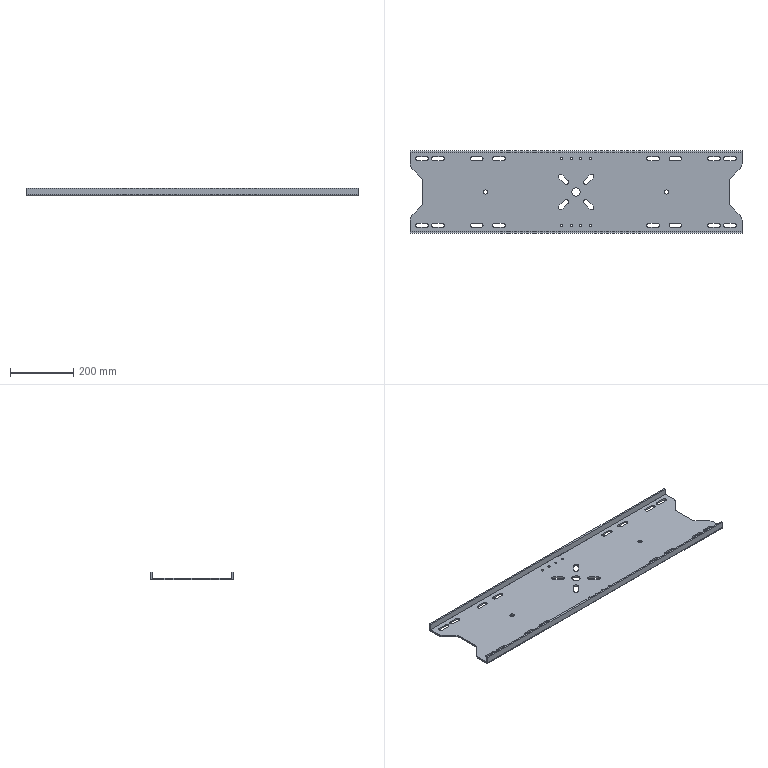Part | SolidWorks | features ICE 6, Fillet 1, FlatPattern 1, SMBaseFlange 1, SheetMetal 1 | 1 solid | 160 faces | box 1046 x 260 x 25 mm | volume 1454749 mm3 | cylinder 94 | plane 66 | commonest cylinder face diameters 13 x52 7 x16 14 x12 40 x8 0.2 x2 10.2 x2